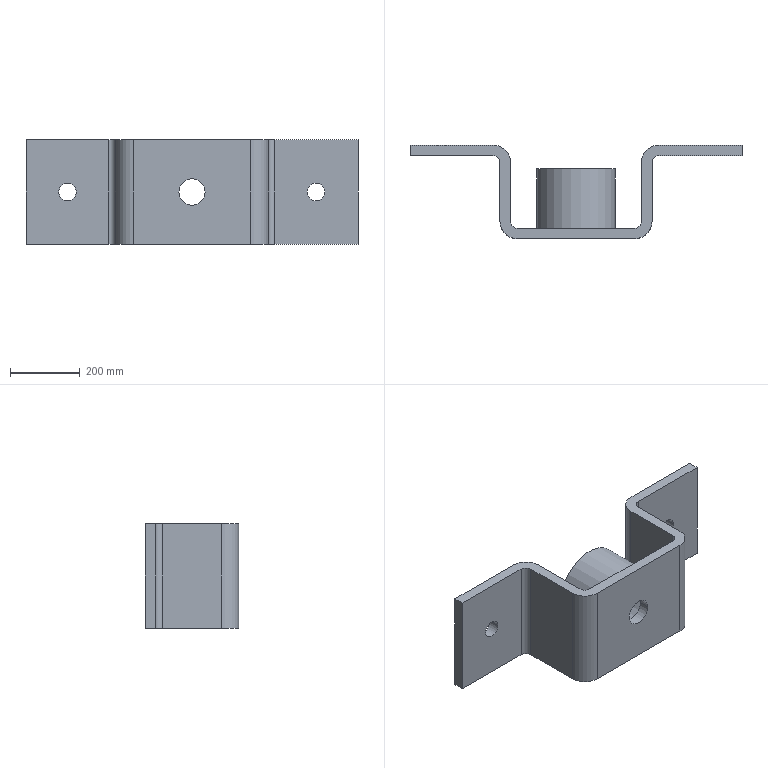Part | SolidWorks | features Fillet 3, ICE 3, Extrusion 1 | 1 solid | 34 faces | box 950 x 268 x 300 mm | volume 14713211 mm3 | cylinder 18 | plane 16 | commonest cylinder face diameters 40 x4 50 x4 100 x4 75 x2 175 x2 225 x2
STEP:
#1=CARTESIAN_POINT('',(330.,208.,150.));
#2=VERTEX_POINT('',#1);
#3=CARTESIAN_POINT('',(380.,208.,150.));
#4=VERTEX_POINT('',#3);
#5=CARTESIAN_POINT('',(355.,208.,150.));
#6=DIRECTION('',(0.,-1.,0.));
#7=DIRECTION('',(0.,0.,1.));
#8=AXIS2_PLACEMENT_3D('',#5,#6,#7);
#9=CIRCLE('',#8,25.);
#10=EDGE_CURVE('',#2,#4,#9,.T.);
#11=ORIENTED_EDGE('',*,*,#10,.T.);
#12=CARTESIAN_POINT('',(380.,238.,150.));
#13=VERTEX_POINT('',#12);
#14=CARTESIAN_POINT('',(380.,-30.001,150.));
#15=DIRECTION('',(0.,1.,0.));
#16=VECTOR('',#15,1000.);
#17=LINE('',#14,#16);
#18=EDGE_CURVE('',#4,#13,#17,.T.);
#19=ORIENTED_EDGE('',*,*,#18,.T.);
#20=CARTESIAN_POINT('',(330.,238.,150.));
#21=VERTEX_POINT('',#20);
#22=CARTESIAN_POINT('',(355.,238.,150.));
#23=DIRECTION('',(0.,1.,0.));
#24=DIRECTION('',(-1.,0.,0.));
#25=AXIS2_PLACEMENT_3D('',#22,#23,#24);
#26=CIRCLE('',#25,25.);
#27=EDGE_CURVE('',#13,#21,#26,.T.);
#28=ORIENTED_EDGE('',*,*,#27,.T.);
#29=CARTESIAN_POINT('',(330.,-30.001,150.));
#30=DIRECTION('',(0.,1.,0.));
#31=VECTOR('',#30,1000.);
#32=LINE('',#29,#31);
#33=EDGE_CURVE('',#2,#21,#32,.T.);
#34=ORIENTED_EDGE('',*,*,#33,.F.);
#35=EDGE_LOOP('',(#11,#19,#28,#34));
#36=FACE_OUTER_BOUND('',#35,.T.);
#37=CARTESIAN_POINT('',(355.,-30.001,150.));
#38=DIRECTION('',(0.,1.,0.));
#39=DIRECTION('',(-1.,0.,0.));
#40=AXIS2_PLACEMENT_3D('',#37,#38,#39);
#41=CYLINDRICAL_SURFACE('',#40,25.);
#42=ADVANCED_FACE('',(#36),#41,.F.);
#43=CARTESIAN_POINT('',(-381.25,208.,150.));
#44=VERTEX_POINT('',#43);
#45=CARTESIAN_POINT('',(-331.25,208.,150.));
#46=VERTEX_POINT('',#45);
#47=CARTESIAN_POINT('',(-356.25,208.,150.));
#48=DIRECTION('',(0.,-1.,0.));
#49=DIRECTION('',(0.,0.,1.));
#50=AXIS2_PLACEMENT_3D('',#47,#48,#49);
#51=CIRCLE('',#50,25.);
#52=EDGE_CURVE('',#44,#46,#51,.T.);
#53=ORIENTED_EDGE('',*,*,#52,.T.);
#54=CARTESIAN_POINT('',(-331.25,238.,150.));
#55=VERTEX_POINT('',#54);
#56=CARTESIAN_POINT('',(-331.25,-30.001,150.));
#57=DIRECTION('',(0.,1.,0.));
#58=VECTOR('',#57,1000.);
#59=LINE('',#56,#58);
#60=EDGE_CURVE('',#46,#55,#59,.T.);
#61=ORIENTED_EDGE('',*,*,#60,.T.);
#62=CARTESIAN_POINT('',(-381.25,238.,150.));
#63=VERTEX_POINT('',#62);
#64=CARTESIAN_POINT('',(-356.25,238.,150.));
#65=DIRECTION('',(0.,1.,0.));
#66=DIRECTION('',(-1.,0.,0.));
#67=AXIS2_PLACEMENT_3D('',#64,#65,#66);
#68=CIRCLE('',#67,25.);
#69=EDGE_CURVE('',#55,#63,#68,.T.);
#70=ORIENTED_EDGE('',*,*,#69,.T.);
#71=CARTESIAN_POINT('',(-381.25,-30.001,150.));
#72=DIRECTION('',(0.,1.,0.));
#73=VECTOR('',#72,1000.);
#74=LINE('',#71,#73);
#75=EDGE_CURVE('',#44,#63,#74,.T.);
#76=ORIENTED_EDGE('',*,*,#75,.F.);
#77=EDGE_LOOP('',(#53,#61,#70,#76));
#78=FACE_OUTER_BOUND('',#77,.T.);
#79=CARTESIAN_POINT('',(-356.25,-30.001,150.));
#80=DIRECTION('',(0.,1.,0.));
#81=DIRECTION('',(-1.,0.,0.));
#82=AXIS2_PLACEMENT_3D('',#79,#80,#81);
#83=CYLINDRICAL_SURFACE('',#82,25.);
#84=ADVANCED_FACE('',(#78),#83,.F.);
#85=CARTESIAN_POINT('',(-37.5,-30.,150.));
#86=VERTEX_POINT('',#85);
#87=CARTESIAN_POINT('',(37.5,-30.,150.));
#88=VERTEX_POINT('',#87);
#89=CARTESIAN_POINT('',(0.,-30.,150.));
#90=DIRECTION('',(0.,-1.,0.));
#91=DIRECTION('',(-1.,0.,0.));
#92=AXIS2_PLACEMENT_3D('',#89,#90,#91);
#93=CIRCLE('',#92,37.5);
#94=EDGE_CURVE('',#86,#88,#93,.T.);
#95=ORIENTED_EDGE('',*,*,#94,.T.);
#96=CARTESIAN_POINT('',(37.5,0.,150.));
#97=VERTEX_POINT('',#96);
#98=CARTESIAN_POINT('',(37.5,-30.001,150.));
#99=DIRECTION('',(0.,1.,0.));
#100=VECTOR('',#99,1000.);
#101=LINE('',#98,#100);
#102=EDGE_CURVE('',#88,#97,#101,.T.);
#103=ORIENTED_EDGE('',*,*,#102,.T.);
#104=CARTESIAN_POINT('',(-37.5,0.,150.));
#105=VERTEX_POINT('',#104);
#106=CARTESIAN_POINT('',(0.,0.,150.));
#107=DIRECTION('',(0.,1.,0.));
#108=DIRECTION('',(-1.,0.,0.));
#109=AXIS2_PLACEMENT_3D('',#106,#107,#108);
#110=CIRCLE('',#109,37.5);
#111=EDGE_CURVE('',#97,#105,#110,.T.);
#112=ORIENTED_EDGE('',*,*,#111,.T.);
#113=CARTESIAN_POINT('',(-37.5,-30.001,150.));
#114=DIRECTION('',(0.,1.,0.));
#115=VECTOR('',#114,1000.);
#116=LINE('',#113,#115);
#117=EDGE_CURVE('',#86,#105,#116,.T.);
#118=ORIENTED_EDGE('',*,*,#117,.F.);
#119=EDGE_LOOP('',(#95,#103,#112,#118));
#120=FACE_OUTER_BOUND('',#119,.T.);
#121=CARTESIAN_POINT('',(0.,-30.001,150.));
#122=DIRECTION('',(0.,1.,0.));
#123=DIRECTION('',(-1.,0.,0.));
#124=AXIS2_PLACEMENT_3D('',#121,#122,#123);
#125=CYLINDRICAL_SURFACE('',#124,37.5);
#126=ADVANCED_FACE('',(#120),#125,.F.);
#127=CARTESIAN_POINT('',(87.5,170.,150.));
#128=VERTEX_POINT('',#127);
#129=CARTESIAN_POINT('',(-87.5,170.,150.));
#130=VERTEX_POINT('',#129);
#131=CARTESIAN_POINT('',(0.,170.,150.));
#132=DIRECTION('',(0.,1.,0.));
#133=DIRECTION('',(-1.,0.,0.));
#134=AXIS2_PLACEMENT_3D('',#131,#132,#133);
#135=CIRCLE('',#134,87.5);
#136=EDGE_CURVE('',#128,#130,#135,.T.);
#137=ORIENTED_EDGE('',*,*,#136,.T.);
#138=CARTESIAN_POINT('',(-87.5,0.,150.));
#139=VERTEX_POINT('',#138);
#140=CARTESIAN_POINT('',(-87.5,170.,150.));
#141=DIRECTION('',(0.,-1.,0.));
#142=VECTOR('',#141,1000.);
#143=LINE('',#140,#142);
#144=EDGE_CURVE('',#130,#139,#143,.T.);
#145=ORIENTED_EDGE('',*,*,#144,.T.);
#146=CARTESIAN_POINT('',(87.5,0.,150.));
#147=VERTEX_POINT('',#146);
#148=CARTESIAN_POINT('',(0.,0.,150.));
#149=DIRECTION('',(0.,1.,0.));
#150=DIRECTION('',(-1.,0.,0.));
#151=AXIS2_PLACEMENT_3D('',#148,#149,#150);
#152=CIRCLE('',#151,87.5);
#153=EDGE_CURVE('',#147,#139,#152,.T.);
#154=ORIENTED_EDGE('',*,*,#153,.F.);
#155=CARTESIAN_POINT('',(87.5,170.,150.));
#156=DIRECTION('',(0.,-1.,0.));
#157=VECTOR('',#156,1000.);
#158=LINE('',#155,#157);
#159=EDGE_CURVE('',#128,#147,#158,.T.);
#160=ORIENTED_EDGE('',*,*,#159,.F.);
#161=EDGE_LOOP('',(#137,#145,#154,#160));
#162=FACE_OUTER_BOUND('',#161,.T.);
#163=CARTESIAN_POINT('',(0.,170.,150.));
#164=DIRECTION('',(0.,-1.,0.));
#165=DIRECTION('',(1.,0.,0.));
#166=AXIS2_PLACEMENT_3D('',#163,#164,#165);
#167=CYLINDRICAL_SURFACE('',#166,87.5);
#168=ADVANCED_FACE('',(#162),#167,.F.);
#169=CARTESIAN_POINT('',(-112.5,170.,150.));
#170=VERTEX_POINT('',#169);
#171=CARTESIAN_POINT('',(112.5,170.,150.));
#172=VERTEX_POINT('',#171);
#173=CARTESIAN_POINT('',(0.,170.,150.));
#174=DIRECTION('',(0.,1.,0.));
#175=DIRECTION('',(-1.,0.,0.));
#176=AXIS2_PLACEMENT_3D('',#173,#174,#175);
#177=CIRCLE('',#176,112.5);
#178=EDGE_CURVE('',#170,#172,#177,.T.);
#179=ORIENTED_EDGE('',*,*,#178,.F.);
#180=CARTESIAN_POINT('',(-112.5,0.,150.));
#181=VERTEX_POINT('',#180);
#182=CARTESIAN_POINT('',(-112.5,170.,150.));
#183=DIRECTION('',(0.,-1.,0.));
#184=VECTOR('',#183,1000.);
#185=LINE('',#182,#184);
#186=EDGE_CURVE('',#170,#181,#185,.T.);
#187=ORIENTED_EDGE('',*,*,#186,.T.);
#188=CARTESIAN_POINT('',(112.5,0.,150.));
#189=VERTEX_POINT('',#188);
#190=CARTESIAN_POINT('',(0.,0.,150.));
#191=DIRECTION('',(0.,1.,0.));
#192=DIRECTION('',(1.,0.,0.));
#193=AXIS2_PLACEMENT_3D('',#190,#191,#192);
#194=CIRCLE('',#193,112.5);
#195=EDGE_CURVE('',#181,#189,#194,.T.);
#196=ORIENTED_EDGE('',*,*,#195,.T.);
#197=CARTESIAN_POINT('',(112.5,170.,150.));
#198=DIRECTION('',(0.,-1.,0.));
#199=VECTOR('',#198,1000.);
#200=LINE('',#197,#199);
#201=EDGE_CURVE('',#172,#189,#200,.T.);
#202=ORIENTED_EDGE('',*,*,#201,.F.);
#203=EDGE_LOOP('',(#179,#187,#196,#202));
#204=FACE_OUTER_BOUND('',#203,.T.);
#205=CARTESIAN_POINT('',(0.,170.,150.));
#206=DIRECTION('',(0.,-1.,0.));
#207=DIRECTION('',(1.,0.,0.));
#208=AXIS2_PLACEMENT_3D('',#205,#206,#207);
#209=CYLINDRICAL_SURFACE('',#208,112.5);
#210=ADVANCED_FACE('',(#204),#209,.T.);
#211=CARTESIAN_POINT('',(167.5,0.,300.));
#212=VERTEX_POINT('',#211);
#213=CARTESIAN_POINT('',(-167.5,0.,300.));
#214=VERTEX_POINT('',#213);
#215=CARTESIAN_POINT('',(187.5,0.,300.));
#216=DIRECTION('',(-1.,0.,0.));
#217=VECTOR('',#216,1000.);
#218=LINE('',#215,#217);
#219=EDGE_CURVE('',#212,#214,#218,.T.);
#220=ORIENTED_EDGE('',*,*,#219,.F.);
#221=CARTESIAN_POINT('',(167.5,0.,0.));
#222=VERTEX_POINT('',#221);
#223=CARTESIAN_POINT('',(167.5,0.,0.));
#224=DIRECTION('',(0.,0.,-1.));
#225=VECTOR('',#224,1000.);
#226=LINE('',#223,#225);
#227=EDGE_CURVE('',#212,#222,#226,.T.);
#228=ORIENTED_EDGE('',*,*,#227,.T.);
#229=CARTESIAN_POINT('',(-167.5,0.,0.));
#230=VERTEX_POINT('',#229);
#231=CARTESIAN_POINT('',(187.5,0.,0.));
#232=DIRECTION('',(-1.,0.,0.));
#233=VECTOR('',#232,1000.);
#234=LINE('',#231,#233);
#235=EDGE_CURVE('',#222,#230,#234,.T.);
#236=ORIENTED_EDGE('',*,*,#235,.T.);
#237=CARTESIAN_POINT('',(-167.5,0.,300.));
#238=DIRECTION('',(0.,0.,1.));
#239=VECTOR('',#238,1000.);
#240=LINE('',#237,#239);
#241=EDGE_CURVE('',#230,#214,#240,.T.);
#242=ORIENTED_EDGE('',*,*,#241,.T.);
#243=EDGE_LOOP('',(#220,#228,#236,#242));
#244=FACE_OUTER_BOUND('',#243,.T.);
#245=CARTESIAN_POINT('',(0.,0.,150.));
#246=DIRECTION('',(0.,1.,0.));
#247=DIRECTION('',(1.,0.,0.));
#248=AXIS2_PLACEMENT_3D('',#245,#246,#247);
#249=CIRCLE('',#248,112.5);
#250=EDGE_CURVE('',#189,#181,#249,.T.);
#251=ORIENTED_EDGE('',*,*,#250,.F.);
#252=ORIENTED_EDGE('',*,*,#195,.F.);
#253=EDGE_LOOP('',(#251,#252));
#254=FACE_BOUND('',#253,.T.);
#255=CARTESIAN_POINT('',(187.5,0.,300.));
#256=DIRECTION('',(0.,-1.,0.));
#257=DIRECTION('',(1.,0.,0.));
#258=AXIS2_PLACEMENT_3D('',#255,#256,#257);
#259=PLANE('',#258);
#260=ADVANCED_FACE('',(#244,#254),#259,.F.);
#261=CARTESIAN_POINT('',(-187.5,20.,0.));
#262=VERTEX_POINT('',#261);
#263=CARTESIAN_POINT('',(-187.5,188.,0.));
#264=VERTEX_POINT('',#263);
#265=CARTESIAN_POINT('',(-187.5,0.,0.));
#266=DIRECTION('',(0.,1.,0.));
#267=VECTOR('',#266,1000.);
#268=LINE('',#265,#267);
#269=EDGE_CURVE('',#262,#264,#268,.T.);
#270=ORIENTED_EDGE('',*,*,#269,.T.);
#271=CARTESIAN_POINT('',(-187.5,188.,300.));
#272=VERTEX_POINT('',#271);
#273=CARTESIAN_POINT('',(-187.5,188.,300.));
#274=DIRECTION('',(0.,0.,1.));
#275=VECTOR('',#274,1000.);
#276=LINE('',#273,#275);
#277=EDGE_CURVE('',#264,#272,#276,.T.);
#278=ORIENTED_EDGE('',*,*,#277,.T.);
#279=CARTESIAN_POINT('',(-187.5,20.,300.));
#280=VERTEX_POINT('',#279);
#281=CARTESIAN_POINT('',(-187.5,0.,300.));
#282=DIRECTION('',(0.,1.,0.));
#283=VECTOR('',#282,1000.);
#284=LINE('',#281,#283);
#285=EDGE_CURVE('',#280,#272,#284,.T.);
#286=ORIENTED_EDGE('',*,*,#285,.F.);
#287=CARTESIAN_POINT('',(-187.5,20.,0.));
#288=DIRECTION('',(0.,0.,-1.));
#289=VECTOR('',#288,1000.);
#290=LINE('',#287,#289);
#291=EDGE_CURVE('',#280,#262,#290,.T.);
#292=ORIENTED_EDGE('',*,*,#291,.T.);
#293=EDGE_LOOP('',(#270,#278,#286,#292));
#294=FACE_OUTER_BOUND('',#293,.T.);
#295=CARTESIAN_POINT('',(-187.5,0.,300.));
#296=DIRECTION('',(-1.,0.,0.));
#297=DIRECTION('',(0.,0.,1.));
#298=AXIS2_PLACEMENT_3D('',#295,#296,#297);
#299=PLANE('',#298);
#300=ADVANCED_FACE('',(#294),#299,.F.);
#301=CARTESIAN_POINT('',(-356.25,238.,150.));
#302=DIRECTION('',(0.,1.,0.));
#303=DIRECTION('',(-1.,0.,0.));
#304=AXIS2_PLACEMENT_3D('',#301,#302,#303);
#305=CIRCLE('',#304,25.);
#306=EDGE_CURVE('',#63,#55,#305,.T.);
#307=ORIENTED_EDGE('',*,*,#306,.F.);
#308=ORIENTED_EDGE('',*,*,#69,.F.);
#309=EDGE_LOOP('',(#307,#308));
#310=FACE_BOUND('',#309,.T.);
#311=CARTESIAN_POINT('',(-237.5,238.,300.));
#312=VERTEX_POINT('',#311);
#313=CARTESIAN_POINT('',(-475.,238.,300.));
#314=VERTEX_POINT('',#313);
#315=CARTESIAN_POINT('',(-187.5,238.,300.));
#316=DIRECTION('',(-1.,0.,0.));
#317=VECTOR('',#316,1000.);
#318=LINE('',#315,#317);
#319=EDGE_CURVE('',#312,#314,#318,.T.);
#320=ORIENTED_EDGE('',*,*,#319,.F.);
#321=CARTESIAN_POINT('',(-237.5,238.,0.));
#322=VERTEX_POINT('',#321);
#323=CARTESIAN_POINT('',(-237.5,238.,300.));
#324=DIRECTION('',(0.,0.,-1.));
#325=VECTOR('',#324,1000.);
#326=LINE('',#323,#325);
#327=EDGE_CURVE('',#312,#322,#326,.T.);
#328=ORIENTED_EDGE('',*,*,#327,.T.);
#329=CARTESIAN_POINT('',(-475.,238.,0.));
#330=VERTEX_POINT('',#329);
#331=CARTESIAN_POINT('',(-187.5,238.,0.));
#332=DIRECTION('',(-1.,0.,0.));
#333=VECTOR('',#332,1000.);
#334=LINE('',#331,#333);
#335=EDGE_CURVE('',#322,#330,#334,.T.);
#336=ORIENTED_EDGE('',*,*,#335,.T.);
#337=CARTESIAN_POINT('',(-475.,238.,300.));
#338=DIRECTION('',(0.,0.,-1.));
#339=VECTOR('',#338,1000.);
#340=LINE('',#337,#339);
#341=EDGE_CURVE('',#314,#330,#340,.T.);
#342=ORIENTED_EDGE('',*,*,#341,.F.);
#343=EDGE_LOOP('',(#320,#328,#336,#342));
#344=FACE_OUTER_BOUND('',#343,.T.);
#345=CARTESIAN_POINT('',(-187.5,238.,300.));
#346=DIRECTION('',(0.,-1.,0.));
#347=DIRECTION('',(1.,0.,0.));
#348=AXIS2_PLACEMENT_3D('',#345,#346,#347);
#349=PLANE('',#348);
#350=ADVANCED_FACE('',(#310,#344),#349,.F.);
#351=CARTESIAN_POINT('',(-475.,208.,0.));
#352=VERTEX_POINT('',#351);
#353=CARTESIAN_POINT('',(-475.,238.,0.));
#354=DIRECTION('',(0.,-1.,0.));
#355=VECTOR('',#354,1000.);
#356=LINE('',#353,#355);
#357=EDGE_CURVE('',#330,#352,#356,.T.);
#358=ORIENTED_EDGE('',*,*,#357,.T.);
#359=CARTESIAN_POINT('',(-475.,208.,300.));
#360=VERTEX_POINT('',#359);
#361=CARTESIAN_POINT('',(-475.,208.,300.));
#362=DIRECTION('',(0.,0.,-1.));
#363=VECTOR('',#362,1000.);
#364=LINE('',#361,#363);
#365=EDGE_CURVE('',#360,#352,#364,.T.);
#366=ORIENTED_EDGE('',*,*,#365,.F.);
#367=CARTESIAN_POINT('',(-475.,238.,300.));
#368=DIRECTION('',(0.,-1.,0.));
#369=VECTOR('',#368,1000.);
#370=LINE('',#367,#369);
#371=EDGE_CURVE('',#314,#360,#370,.T.);
#372=ORIENTED_EDGE('',*,*,#371,.F.);
#373=ORIENTED_EDGE('',*,*,#341,.T.);
#374=EDGE_LOOP('',(#358,#366,#372,#373));
#375=FACE_OUTER_BOUND('',#374,.T.);
#376=CARTESIAN_POINT('',(-475.,238.,300.));
#377=DIRECTION('',(1.,0.,0.));
#378=DIRECTION('',(0.,0.,-1.));
#379=AXIS2_PLACEMENT_3D('',#376,#377,#378);
#380=PLANE('',#379);
#381=ADVANCED_FACE('',(#375),#380,.F.);
#382=ORIENTED_EDGE('',*,*,#52,.F.);
#383=CARTESIAN_POINT('',(-356.25,208.,150.));
#384=DIRECTION('',(0.,-1.,0.));
#385=DIRECTION('',(0.,0.,1.));
#386=AXIS2_PLACEMENT_3D('',#383,#384,#385);
#387=CIRCLE('',#386,25.);
#388=EDGE_CURVE('',#46,#44,#387,.T.);
#389=ORIENTED_EDGE('',*,*,#388,.F.);
#390=EDGE_LOOP('',(#382,#389));
#391=FACE_BOUND('',#390,.T.);
#392=CARTESIAN_POINT('',(-237.5,208.,0.));
#393=VERTEX_POINT('',#392);
#394=CARTESIAN_POINT('',(-475.,208.,0.));
#395=DIRECTION('',(1.,0.,0.));
#396=VECTOR('',#395,1000.);
#397=LINE('',#394,#396);
#398=EDGE_CURVE('',#352,#393,#397,.T.);
#399=ORIENTED_EDGE('',*,*,#398,.T.);
#400=CARTESIAN_POINT('',(-237.5,208.,300.));
#401=VERTEX_POINT('',#400);
#402=CARTESIAN_POINT('',(-237.5,208.,300.));
#403=DIRECTION('',(0.,0.,1.));
#404=VECTOR('',#403,1000.);
#405=LINE('',#402,#404);
#406=EDGE_CURVE('',#393,#401,#405,.T.);
#407=ORIENTED_EDGE('',*,*,#406,.T.);
#408=CARTESIAN_POINT('',(-475.,208.,300.));
#409=DIRECTION('',(1.,0.,0.));
#410=VECTOR('',#409,1000.);
#411=LINE('',#408,#410);
#412=EDGE_CURVE('',#360,#401,#411,.T.);
#413=ORIENTED_EDGE('',*,*,#412,.F.);
#414=ORIENTED_EDGE('',*,*,#365,.T.);
#415=EDGE_LOOP('',(#399,#407,#413,#414));
#416=FACE_OUTER_BOUND('',#415,.T.);
#417=CARTESIAN_POINT('',(-475.,208.,300.));
#418=DIRECTION('',(0.,1.,0.));
#419=DIRECTION('',(0.,0.,1.));
#420=AXIS2_PLACEMENT_3D('',#417,#418,#419);
#421=PLANE('',#420);
#422=ADVANCED_FACE('',(#391,#416),#421,.F.);
#423=CARTESIAN_POINT('',(-217.5,188.,300.));
#424=VERTEX_POINT('',#423);
#425=CARTESIAN_POINT('',(-217.5,20.,300.));
#426=VERTEX_POINT('',#425);
#427=CARTESIAN_POINT('',(-217.5,208.,300.));
#428=DIRECTION('',(0.,-1.,0.));
#429=VECTOR('',#428,1000.);
#430=LINE('',#427,#429);
#431=EDGE_CURVE('',#424,#426,#430,.T.);
#432=ORIENTED_EDGE('',*,*,#431,.F.);
#433=CARTESIAN_POINT('',(-217.5,188.,0.));
#434=VERTEX_POINT('',#433);
#435=CARTESIAN_POINT('',(-217.5,188.,0.));
#436=DIRECTION('',(0.,0.,-1.));
#437=VECTOR('',#436,1000.);
#438=LINE('',#435,#437);
#439=EDGE_CURVE('',#424,#434,#438,.T.);
#440=ORIENTED_EDGE('',*,*,#439,.T.);
#441=CARTESIAN_POINT('',(-217.5,20.,0.));
#442=VERTEX_POINT('',#441);
#443=CARTESIAN_POINT('',(-217.5,208.,0.));
#444=DIRECTION('',(0.,-1.,0.));
#445=VECTOR('',#444,1000.);
#446=LINE('',#443,#445);
#447=EDGE_CURVE('',#434,#442,#446,.T.);
#448=ORIENTED_EDGE('',*,*,#447,.T.);
#449=CARTESIAN_POINT('',(-217.5,20.,300.));
#450=DIRECTION('',(0.,0.,1.));
#451=VECTOR('',#450,1000.);
#452=LINE('',#449,#451);
#453=EDGE_CURVE('',#442,#426,#452,.T.);
#454=ORIENTED_EDGE('',*,*,#453,.T.);
#455=EDGE_LOOP('',(#432,#440,#448,#454));
#456=FACE_OUTER_BOUND('',#455,.T.);
#457=CARTESIAN_POINT('',(-217.5,208.,300.));
#458=DIRECTION('',(1.,0.,0.));
#459=DIRECTION('',(0.,1.,0.));
#460=AXIS2_PLACEMENT_3D('',#457,#458,#459);
#461=PLANE('',#460);
#462=ADVANCED_FACE('',(#456),#461,.F.);
#463=ORIENTED_EDGE('',*,*,#94,.F.);
#464=CARTESIAN_POINT('',(0.,-30.,150.));
#465=DIRECTION('',(0.,-1.,0.));
#466=DIRECTION('',(-1.,0.,0.));
#467=AXIS2_PLACEMENT_3D('',#464,#465,#466);
#468=CIRCLE('',#467,37.5);
#469=EDGE_CURVE('',#88,#86,#468,.T.);
#470=ORIENTED_EDGE('',*,*,#469,.F.);
#471=EDGE_LOOP('',(#463,#470));
#472=FACE_BOUND('',#471,.T.);
#473=CARTESIAN_POINT('',(-167.5,-30.,0.));
#474=VERTEX_POINT('',#473);
#475=CARTESIAN_POINT('',(167.5,-30.,0.));
#476=VERTEX_POINT('',#475);
#477=CARTESIAN_POINT('',(-217.5,-30.,0.));
#478=DIRECTION('',(1.,0.,0.));
#479=VECTOR('',#478,1000.);
#480=LINE('',#477,#479);
#481=EDGE_CURVE('',#474,#476,#480,.T.);
#482=ORIENTED_EDGE('',*,*,#481,.T.);
#483=CARTESIAN_POINT('',(167.5,-30.,300.));
#484=VERTEX_POINT('',#483);
#485=CARTESIAN_POINT('',(167.5,-30.,300.));
#486=DIRECTION('',(0.,0.,1.));
#487=VECTOR('',#486,1000.);
#488=LINE('',#485,#487);
#489=EDGE_CURVE('',#476,#484,#488,.T.);
#490=ORIENTED_EDGE('',*,*,#489,.T.);
#491=CARTESIAN_POINT('',(-167.5,-30.,300.));
#492=VERTEX_POINT('',#491);
#493=CARTESIAN_POINT('',(-217.5,-30.,300.));
#494=DIRECTION('',(1.,0.,0.));
#495=VECTOR('',#494,1000.);
#496=LINE('',#493,#495);
#497=EDGE_CURVE('',#492,#484,#496,.T.);
#498=ORIENTED_EDGE('',*,*,#497,.F.);
#499=CARTESIAN_POINT('',(-167.5,-30.,300.));
#500=DIRECTION('',(0.,0.,-1.));
#501=VECTOR('',#500,1000.);
#502=LINE('',#499,#501);
#503=EDGE_CURVE('',#492,#474,#502,.T.);
#504=ORIENTED_EDGE('',*,*,#503,.T.);
#505=EDGE_LOOP('',(#482,#490,#498,#504));
#506=FACE_OUTER_BOUND('',#505,.T.);
#507=CARTESIAN_POINT('',(-217.5,-30.,300.));
#508=DIRECTION('',(0.,1.,0.));
#509=DIRECTION('',(-1.,0.,0.));
#510=AXIS2_PLACEMENT_3D('',#507,#508,#509);
#511=PLANE('',#510);
#512=ADVANCED_FACE('',(#472,#506),#511,.F.);
#513=CARTESIAN_POINT('',(217.5,20.,0.));
#514=VERTEX_POINT('',#513);
#515=CARTESIAN_POINT('',(217.5,188.,0.));
#516=VERTEX_POINT('',#515);
#517=CARTESIAN_POINT('',(217.5,208.,0.));
#518=DIRECTION('',(0.,1.,0.));
#519=VECTOR('',#518,1000.);
#520=LINE('',#517,#519);
#521=EDGE_CURVE('',#514,#516,#520,.T.);
#522=ORIENTED_EDGE('',*,*,#521,.T.);
#523=CARTESIAN_POINT('',(217.5,188.,300.));
#524=VERTEX_POINT('',#523);
#525=CARTESIAN_POINT('',(217.5,188.,300.));
#526=DIRECTION('',(0.,0.,1.));
#527=VECTOR('',#526,1000.);
#528=LINE('',#525,#527);
#529=EDGE_CURVE('',#516,#524,#528,.T.);
#530=ORIENTED_EDGE('',*,*,#529,.T.);
#531=CARTESIAN_POINT('',(217.5,20.,300.));
#532=VERTEX_POINT('',#531);
#533=CARTESIAN_POINT('',(217.5,208.,300.));
#534=DIRECTION('',(0.,1.,0.));
#535=VECTOR('',#534,1000.);
#536=LINE('',#533,#535);
#537=EDGE_CURVE('',#532,#524,#536,.T.);
#538=ORIENTED_EDGE('',*,*,#537,.F.);
#539=CARTESIAN_POINT('',(217.5,20.,300.));
#540=DIRECTION('',(0.,0.,-1.));
#541=VECTOR('',#540,1000.);
#542=LINE('',#539,#541);
#543=EDGE_CURVE('',#532,#514,#542,.T.);
#544=ORIENTED_EDGE('',*,*,#543,.T.);
#545=EDGE_LOOP('',(#522,#530,#538,#544));
#546=FACE_OUTER_BOUND('',#545,.T.);
#547=CARTESIAN_POINT('',(217.5,208.,300.));
#548=DIRECTION('',(-1.,0.,0.));
#549=DIRECTION('',(0.,-1.,0.));
#550=AXIS2_PLACEMENT_3D('',#547,#548,#549);
#551=PLANE('',#550);
#552=ADVANCED_FACE('',(#546),#551,.F.);
#553=ORIENTED_EDGE('',*,*,#10,.F.);
#554=CARTESIAN_POINT('',(355.,208.,150.));
#555=DIRECTION('',(0.,-1.,0.));
#556=DIRECTION('',(0.,0.,1.));
#557=AXIS2_PLACEMENT_3D('',#554,#555,#556);
#558=CIRCLE('',#557,25.);
#559=EDGE_CURVE('',#4,#2,#558,.T.);
#560=ORIENTED_EDGE('',*,*,#559,.F.);
#561=EDGE_LOOP('',(#553,#560));
#562=FACE_BOUND('',#561,.T.);
#563=CARTESIAN_POINT('',(237.5,208.,300.));
#564=VERTEX_POINT('',#563);
#565=CARTESIAN_POINT('',(475.,208.,300.));
#566=VERTEX_POINT('',#565);
#567=CARTESIAN_POINT('',(475.,208.,300.));
#568=DIRECTION('',(1.,0.,0.));
#569=VECTOR('',#568,1000.);
#570=LINE('',#567,#569);
#571=EDGE_CURVE('',#564,#566,#570,.T.);
#572=ORIENTED_EDGE('',*,*,#571,.F.);
#573=CARTESIAN_POINT('',(237.5,208.,0.));
#574=VERTEX_POINT('',#573);
#575=CARTESIAN_POINT('',(237.5,208.,0.));
#576=DIRECTION('',(0.,0.,-1.));
#577=VECTOR('',#576,1000.);
#578=LINE('',#575,#577);
#579=EDGE_CURVE('',#564,#574,#578,.T.);
#580=ORIENTED_EDGE('',*,*,#579,.T.);
#581=CARTESIAN_POINT('',(475.,208.,0.));
#582=VERTEX_POINT('',#581);
#583=CARTESIAN_POINT('',(475.,208.,0.));
#584=DIRECTION('',(1.,0.,0.));
#585=VECTOR('',#584,1000.);
#586=LINE('',#583,#585);
#587=EDGE_CURVE('',#574,#582,#586,.T.);
#588=ORIENTED_EDGE('',*,*,#587,.T.);
#589=CARTESIAN_POINT('',(475.,208.,300.));
#590=DIRECTION('',(0.,0.,-1.));
#591=VECTOR('',#590,1000.);
#592=LINE('',#589,#591);
#593=EDGE_CURVE('',#566,#582,#592,.T.);
#594=ORIENTED_EDGE('',*,*,#593,.F.);
#595=EDGE_LOOP('',(#572,#580,#588,#594));
#596=FACE_OUTER_BOUND('',#595,.T.);
#597=CARTESIAN_POINT('',(475.,208.,300.));
#598=DIRECTION('',(0.,1.,0.));
#599=DIRECTION('',(0.,0.,1.));
#600=AXIS2_PLACEMENT_3D('',#597,#598,#599);
#601=PLANE('',#600);
#602=ADVANCED_FACE('',(#562,#596),#601,.F.);
#603=CARTESIAN_POINT('',(475.,238.,0.));
#604=VERTEX_POINT('',#603);
#605=CARTESIAN_POINT('',(475.,238.,0.));
#606=DIRECTION('',(0.,1.,0.));
#607=VECTOR('',#606,1000.);
#608=LINE('',#605,#607);
#609=EDGE_CURVE('',#582,#604,#608,.T.);
#610=ORIENTED_EDGE('',*,*,#609,.T.);
#611=CARTESIAN_POINT('',(475.,238.,300.));
#612=VERTEX_POINT('',#611);
#613=CARTESIAN_POINT('',(475.,238.,300.));
#614=DIRECTION('',(0.,0.,-1.));
#615=VECTOR('',#614,1000.);
#616=LINE('',#613,#615);
#617=EDGE_CURVE('',#612,#604,#616,.T.);
#618=ORIENTED_EDGE('',*,*,#617,.F.);
#619=CARTESIAN_POINT('',(475.,238.,300.));
#620=DIRECTION('',(0.,1.,0.));
#621=VECTOR('',#620,1000.);
#622=LINE('',#619,#621);
#623=EDGE_CURVE('',#566,#612,#622,.T.);
#624=ORIENTED_EDGE('',*,*,#623,.F.);
#625=ORIENTED_EDGE('',*,*,#593,.T.);
#626=EDGE_LOOP('',(#610,#618,#624,#625));
#627=FACE_OUTER_BOUND('',#626,.T.);
#628=CARTESIAN_POINT('',(475.,238.,300.));
#629=DIRECTION('',(-1.,0.,0.));
#630=DIRECTION('',(0.,0.,1.));
#631=AXIS2_PLACEMENT_3D('',#628,#629,#630);
#632=PLANE('',#631);
#633=ADVANCED_FACE('',(#627),#632,.F.);
#634=CARTESIAN_POINT('',(355.,238.,150.));
#635=DIRECTION('',(0.,1.,0.));
#636=DIRECTION('',(-1.,0.,0.));
#637=AXIS2_PLACEMENT_3D('',#634,#635,#636);
#638=CIRCLE('',#637,25.);
#639=EDGE_CURVE('',#21,#13,#638,.T.);
#640=ORIENTED_EDGE('',*,*,#639,.F.);
#641=ORIENTED_EDGE('',*,*,#27,.F.);
#642=EDGE_LOOP('',(#640,#641));
#643=FACE_BOUND('',#642,.T.);
#644=CARTESIAN_POINT('',(237.5,238.,0.));
#645=VERTEX_POINT('',#644);
#646=CARTESIAN_POINT('',(187.5,238.,0.));
#647=DIRECTION('',(-1.,0.,0.));
#648=VECTOR('',#647,1000.);
#649=LINE('',#646,#648);
#650=EDGE_CURVE('',#604,#645,#649,.T.);
#651=ORIENTED_EDGE('',*,*,#650,.T.);
#652=CARTESIAN_POINT('',(237.5,238.,300.));
#653=VERTEX_POINT('',#652);
#654=CARTESIAN_POINT('',(237.5,238.,300.));
#655=DIRECTION('',(0.,0.,1.));
#656=VECTOR('',#655,1000.);
#657=LINE('',#654,#656);
#658=EDGE_CURVE('',#645,#653,#657,.T.);
#659=ORIENTED_EDGE('',*,*,#658,.T.);
#660=CARTESIAN_POINT('',(187.5,238.,300.));
#661=DIRECTION('',(-1.,0.,0.));
#662=VECTOR('',#661,1000.);
#663=LINE('',#660,#662);
#664=EDGE_CURVE('',#612,#653,#663,.T.);
#665=ORIENTED_EDGE('',*,*,#664,.F.);
#666=ORIENTED_EDGE('',*,*,#617,.T.);
#667=EDGE_LOOP('',(#651,#659,#665,#666));
#668=FACE_OUTER_BOUND('',#667,.T.);
#669=CARTESIAN_POINT('',(187.5,238.,300.));
#670=DIRECTION('',(0.,-1.,0.));
#671=DIRECTION('',(1.,0.,0.));
#672=AXIS2_PLACEMENT_3D('',#669,#670,#671);
#673=PLANE('',#672);
#674=ADVANCED_FACE('',(#643,#668),#673,.F.);
#675=CARTESIAN_POINT('',(187.5,188.,300.));
#676=VERTEX_POINT('',#675);
#677=CARTESIAN_POINT('',(187.5,20.,300.));
#678=VERTEX_POINT('',#677);
#679=CARTESIAN_POINT('',(187.5,0.,300.));
#680=DIRECTION('',(0.,-1.,0.));
#681=VECTOR('',#680,1000.);
#682=LINE('',#679,#681);
#683=EDGE_CURVE('',#676,#678,#682,.T.);
#684=ORIENTED_EDGE('',*,*,#683,.F.);
#685=CARTESIAN_POINT('',(187.5,188.,0.));
#686=VERTEX_POINT('',#685);
#687=CARTESIAN_POINT('',(187.5,188.,300.));
#688=DIRECTION('',(0.,0.,-1.));
#689=VECTOR('',#688,1000.);
#690=LINE('',#687,#689);
#691=EDGE_CURVE('',#676,#686,#690,.T.);
#692=ORIENTED_EDGE('',*,*,#691,.T.);
#693=CARTESIAN_POINT('',(187.5,20.,0.));
#694=VERTEX_POINT('',#693);
#695=CARTESIAN_POINT('',(187.5,0.,0.));
#696=DIRECTION('',(0.,-1.,0.));
#697=VECTOR('',#696,1000.);
#698=LINE('',#695,#697);
#699=EDGE_CURVE('',#686,#694,#698,.T.);
#700=ORIENTED_EDGE('',*,*,#699,.T.);
#701=CARTESIAN_POINT('',(187.5,20.,300.));
#702=DIRECTION('',(0.,0.,1.));
#703=VECTOR('',#702,1000.);
#704=LINE('',#701,#703);
#705=EDGE_CURVE('',#694,#678,#704,.T.);
#706=ORIENTED_EDGE('',*,*,#705,.T.);
#707=EDGE_LOOP('',(#684,#692,#700,#706));
#708=FACE_OUTER_BOUND('',#707,.T.);
#709=CARTESIAN_POINT('',(187.5,0.,300.));
#710=DIRECTION('',(1.,0.,0.));
#711=DIRECTION('',(0.,0.,-1.));
#712=AXIS2_PLACEMENT_3D('',#709,#710,#711);
#713=PLANE('',#712);
#714=ADVANCED_FACE('',(#708),#713,.F.);
#715=ORIENTED_EDGE('',*,*,#497,.T.);
#716=CARTESIAN_POINT('',(167.5,20.,300.));
#717=DIRECTION('',(0.,0.,1.));
#718=DIRECTION('',(1.,0.,0.));
#719=AXIS2_PLACEMENT_3D('',#716,#717,#718);
#720=CIRCLE('',#719,50.);
#721=EDGE_CURVE('',#484,#532,#720,.T.);
#722=ORIENTED_EDGE('',*,*,#721,.T.);
#723=ORIENTED_EDGE('',*,*,#537,.T.);
#724=CARTESIAN_POINT('',(237.5,188.,300.));
#725=DIRECTION('',(0.,0.,-1.));
#726=DIRECTION('',(1.,0.,0.));
#727=AXIS2_PLACEMENT_3D('',#724,#725,#726);
#728=CIRCLE('',#727,20.);
#729=EDGE_CURVE('',#524,#564,#728,.T.);
#730=ORIENTED_EDGE('',*,*,#729,.T.);
#731=ORIENTED_EDGE('',*,*,#571,.T.);
#732=ORIENTED_EDGE('',*,*,#623,.T.);
#733=ORIENTED_EDGE('',*,*,#664,.T.);
#734=CARTESIAN_POINT('',(237.5,188.,300.));
#735=DIRECTION('',(0.,0.,1.));
#736=DIRECTION('',(1.,0.,0.));
#737=AXIS2_PLACEMENT_3D('',#734,#735,#736);
#738=CIRCLE('',#737,50.);
#739=EDGE_CURVE('',#653,#676,#738,.T.);
#740=ORIENTED_EDGE('',*,*,#739,.T.);
#741=ORIENTED_EDGE('',*,*,#683,.T.);
#742=CARTESIAN_POINT('',(167.5,20.,300.));
#743=DIRECTION('',(0.,0.,-1.));
#744=DIRECTION('',(1.,0.,0.));
#745=AXIS2_PLACEMENT_3D('',#742,#743,#744);
#746=CIRCLE('',#745,20.);
#747=EDGE_CURVE('',#678,#212,#746,.T.);
#748=ORIENTED_EDGE('',*,*,#747,.T.);
#749=ORIENTED_EDGE('',*,*,#219,.T.);
#750=CARTESIAN_POINT('',(-167.5,20.,300.));
#751=DIRECTION('',(0.,0.,-1.));
#752=DIRECTION('',(1.,0.,0.));
#753=AXIS2_PLACEMENT_3D('',#750,#751,#752);
#754=CIRCLE('',#753,20.);
#755=EDGE_CURVE('',#214,#280,#754,.T.);
#756=ORIENTED_EDGE('',*,*,#755,.T.);
#757=ORIENTED_EDGE('',*,*,#285,.T.);
#758=CARTESIAN_POINT('',(-237.5,188.,300.));
#759=DIRECTION('',(0.,0.,1.));
#760=DIRECTION('',(1.,0.,0.));
#761=AXIS2_PLACEMENT_3D('',#758,#759,#760);
#762=CIRCLE('',#761,50.);
#763=EDGE_CURVE('',#272,#312,#762,.T.);
#764=ORIENTED_EDGE('',*,*,#763,.T.);
#765=ORIENTED_EDGE('',*,*,#319,.T.);
#766=ORIENTED_EDGE('',*,*,#371,.T.);
#767=ORIENTED_EDGE('',*,*,#412,.T.);
#768=CARTESIAN_POINT('',(-237.5,188.,300.));
#769=DIRECTION('',(0.,0.,-1.));
#770=DIRECTION('',(1.,0.,0.));
#771=AXIS2_PLACEMENT_3D('',#768,#769,#770);
#772=CIRCLE('',#771,20.);
#773=EDGE_CURVE('',#401,#424,#772,.T.);
#774=ORIENTED_EDGE('',*,*,#773,.T.);
#775=ORIENTED_EDGE('',*,*,#431,.T.);
#776=CARTESIAN_POINT('',(-167.5,20.,300.));
#777=DIRECTION('',(0.,0.,1.));
#778=DIRECTION('',(1.,0.,0.));
#779=AXIS2_PLACEMENT_3D('',#776,#777,#778);
#780=CIRCLE('',#779,50.);
#781=EDGE_CURVE('',#426,#492,#780,.T.);
#782=ORIENTED_EDGE('',*,*,#781,.T.);
#783=EDGE_LOOP('',(#715,#722,#723,#730,#731,#732,#733,#740,#741,#748,#749,#756,#757,#764,#765,#766,#767,#774,#775,#782));
#784=FACE_OUTER_BOUND('',#783,.T.);
#785=CARTESIAN_POINT('',(0.,0.,300.));
#786=DIRECTION('',(0.,0.,1.));
#787=DIRECTION('',(1.,0.,0.));
#788=AXIS2_PLACEMENT_3D('',#785,#786,#787);
#789=PLANE('',#788);
#790=ADVANCED_FACE('',(#784),#789,.T.);
#791=ORIENTED_EDGE('',*,*,#521,.F.);
#792=CARTESIAN_POINT('',(167.5,20.,0.));
#793=DIRECTION('',(0.,0.,-1.));
#794=DIRECTION('',(1.,0.,0.));
#795=AXIS2_PLACEMENT_3D('',#792,#793,#794);
#796=CIRCLE('',#795,50.);
#797=EDGE_CURVE('',#514,#476,#796,.T.);
#798=ORIENTED_EDGE('',*,*,#797,.T.);
#799=ORIENTED_EDGE('',*,*,#481,.F.);
#800=CARTESIAN_POINT('',(-167.5,20.,0.));
#801=DIRECTION('',(0.,0.,-1.));
#802=DIRECTION('',(1.,0.,0.));
#803=AXIS2_PLACEMENT_3D('',#800,#801,#802);
#804=CIRCLE('',#803,50.);
#805=EDGE_CURVE('',#474,#442,#804,.T.);
#806=ORIENTED_EDGE('',*,*,#805,.T.);
#807=ORIENTED_EDGE('',*,*,#447,.F.);
#808=CARTESIAN_POINT('',(-237.5,188.,0.));
#809=DIRECTION('',(0.,0.,1.));
#810=DIRECTION('',(1.,0.,0.));
#811=AXIS2_PLACEMENT_3D('',#808,#809,#810);
#812=CIRCLE('',#811,20.);
#813=EDGE_CURVE('',#434,#393,#812,.T.);
#814=ORIENTED_EDGE('',*,*,#813,.T.);
#815=ORIENTED_EDGE('',*,*,#398,.F.);
#816=ORIENTED_EDGE('',*,*,#357,.F.);
#817=ORIENTED_EDGE('',*,*,#335,.F.);
#818=CARTESIAN_POINT('',(-237.5,188.,0.));
#819=DIRECTION('',(0.,0.,-1.));
#820=DIRECTION('',(1.,0.,0.));
#821=AXIS2_PLACEMENT_3D('',#818,#819,#820);
#822=CIRCLE('',#821,50.);
#823=EDGE_CURVE('',#322,#264,#822,.T.);
#824=ORIENTED_EDGE('',*,*,#823,.T.);
#825=ORIENTED_EDGE('',*,*,#269,.F.);
#826=CARTESIAN_POINT('',(-167.5,20.,0.));
#827=DIRECTION('',(0.,0.,1.));
#828=DIRECTION('',(1.,0.,0.));
#829=AXIS2_PLACEMENT_3D('',#826,#827,#828);
#830=CIRCLE('',#829,20.);
#831=EDGE_CURVE('',#262,#230,#830,.T.);
#832=ORIENTED_EDGE('',*,*,#831,.T.);
#833=ORIENTED_EDGE('',*,*,#235,.F.);
#834=CARTESIAN_POINT('',(167.5,20.,0.));
#835=DIRECTION('',(0.,0.,1.));
#836=DIRECTION('',(1.,0.,0.));
#837=AXIS2_PLACEMENT_3D('',#834,#835,#836);
#838=CIRCLE('',#837,20.);
#839=EDGE_CURVE('',#222,#694,#838,.T.);
#840=ORIENTED_EDGE('',*,*,#839,.T.);
#841=ORIENTED_EDGE('',*,*,#699,.F.);
#842=CARTESIAN_POINT('',(237.5,188.,0.));
#843=DIRECTION('',(0.,0.,-1.));
#844=DIRECTION('',(1.,0.,0.));
#845=AXIS2_PLACEMENT_3D('',#842,#843,#844);
#846=CIRCLE('',#845,50.);
#847=EDGE_CURVE('',#686,#645,#846,.T.);
#848=ORIENTED_EDGE('',*,*,#847,.T.);
#849=ORIENTED_EDGE('',*,*,#650,.F.);
#850=ORIENTED_EDGE('',*,*,#609,.F.);
#851=ORIENTED_EDGE('',*,*,#587,.F.);
#852=CARTESIAN_POINT('',(237.5,188.,0.));
#853=DIRECTION('',(0.,0.,1.));
#854=DIRECTION('',(1.,0.,0.));
#855=AXIS2_PLACEMENT_3D('',#852,#853,#854);
#856=CIRCLE('',#855,20.);
#857=EDGE_CURVE('',#574,#516,#856,.T.);
#858=ORIENTED_EDGE('',*,*,#857,.T.);
#859=EDGE_LOOP('',(#791,#798,#799,#806,#807,#814,#815,#816,#817,#824,#825,#832,#833,#840,#841,#848,#849,#850,#851,#858));
#860=FACE_OUTER_BOUND('',#859,.T.);
#861=CARTESIAN_POINT('',(0.,0.,0.));
#862=DIRECTION('',(0.,0.,1.));
#863=DIRECTION('',(1.,0.,0.));
#864=AXIS2_PLACEMENT_3D('',#861,#862,#863);
#865=PLANE('',#864);
#866=ADVANCED_FACE('',(#860),#865,.F.);
#867=ORIENTED_EDGE('',*,*,#747,.F.);
#868=ORIENTED_EDGE('',*,*,#705,.F.);
#869=ORIENTED_EDGE('',*,*,#839,.F.);
#870=ORIENTED_EDGE('',*,*,#227,.F.);
#871=EDGE_LOOP('',(#867,#868,#869,#870));
#872=FACE_OUTER_BOUND('',#871,.T.);
#873=CARTESIAN_POINT('',(167.5,20.,300.));
#874=DIRECTION('',(0.,0.,1.));
#875=DIRECTION('',(1.,0.,0.));
#876=AXIS2_PLACEMENT_3D('',#873,#874,#875);
#877=CYLINDRICAL_SURFACE('',#876,20.);
#878=ADVANCED_FACE('',(#872),#877,.F.);
#879=ORIENTED_EDGE('',*,*,#755,.F.);
#880=ORIENTED_EDGE('',*,*,#241,.F.);
#881=ORIENTED_EDGE('',*,*,#831,.F.);
#882=ORIENTED_EDGE('',*,*,#291,.F.);
#883=EDGE_LOOP('',(#879,#880,#881,#882));
#884=FACE_OUTER_BOUND('',#883,.T.);
#885=CARTESIAN_POINT('',(-167.5,20.,300.));
#886=DIRECTION('',(0.,0.,1.));
#887=DIRECTION('',(1.,0.,0.));
#888=AXIS2_PLACEMENT_3D('',#885,#886,#887);
#889=CYLINDRICAL_SURFACE('',#888,20.);
#890=ADVANCED_FACE('',(#884),#889,.F.);
#891=ORIENTED_EDGE('',*,*,#721,.F.);
#892=ORIENTED_EDGE('',*,*,#489,.F.);
#893=ORIENTED_EDGE('',*,*,#797,.F.);
#894=ORIENTED_EDGE('',*,*,#543,.F.);
#895=EDGE_LOOP('',(#891,#892,#893,#894));
#896=FACE_OUTER_BOUND('',#895,.T.);
#897=CARTESIAN_POINT('',(167.5,20.,300.));
#898=DIRECTION('',(0.,0.,-1.));
#899=DIRECTION('',(-1.,0.,0.));
#900=AXIS2_PLACEMENT_3D('',#897,#898,#899);
#901=CYLINDRICAL_SURFACE('',#900,50.);
#902=ADVANCED_FACE('',(#896),#901,.T.);
#903=ORIENTED_EDGE('',*,*,#781,.F.);
#904=ORIENTED_EDGE('',*,*,#453,.F.);
#905=ORIENTED_EDGE('',*,*,#805,.F.);
#906=ORIENTED_EDGE('',*,*,#503,.F.);
#907=EDGE_LOOP('',(#903,#904,#905,#906));
#908=FACE_OUTER_BOUND('',#907,.T.);
#909=CARTESIAN_POINT('',(-167.5,20.,300.));
#910=DIRECTION('',(0.,0.,-1.));
#911=DIRECTION('',(-1.,0.,0.));
#912=AXIS2_PLACEMENT_3D('',#909,#910,#911);
#913=CYLINDRICAL_SURFACE('',#912,50.);
#914=ADVANCED_FACE('',(#908),#913,.T.);
#915=ORIENTED_EDGE('',*,*,#739,.F.);
#916=ORIENTED_EDGE('',*,*,#658,.F.);
#917=ORIENTED_EDGE('',*,*,#847,.F.);
#918=ORIENTED_EDGE('',*,*,#691,.F.);
#919=EDGE_LOOP('',(#915,#916,#917,#918));
#920=FACE_OUTER_BOUND('',#919,.T.);
#921=CARTESIAN_POINT('',(237.5,188.,300.));
#922=DIRECTION('',(0.,0.,-1.));
#923=DIRECTION('',(-1.,0.,0.));
#924=AXIS2_PLACEMENT_3D('',#921,#922,#923);
#925=CYLINDRICAL_SURFACE('',#924,50.);
#926=ADVANCED_FACE('',(#920),#925,.T.);
#927=ORIENTED_EDGE('',*,*,#763,.F.);
#928=ORIENTED_EDGE('',*,*,#277,.F.);
#929=ORIENTED_EDGE('',*,*,#823,.F.);
#930=ORIENTED_EDGE('',*,*,#327,.F.);
#931=EDGE_LOOP('',(#927,#928,#929,#930));
#932=FACE_OUTER_BOUND('',#931,.T.);
#933=CARTESIAN_POINT('',(-237.5,188.,300.));
#934=DIRECTION('',(0.,0.,-1.));
#935=DIRECTION('',(-1.,0.,0.));
#936=AXIS2_PLACEMENT_3D('',#933,#934,#935);
#937=CYLINDRICAL_SURFACE('',#936,50.);
#938=ADVANCED_FACE('',(#932),#937,.T.);
#939=ORIENTED_EDGE('',*,*,#773,.F.);
#940=ORIENTED_EDGE('',*,*,#406,.F.);
#941=ORIENTED_EDGE('',*,*,#813,.F.);
#942=ORIENTED_EDGE('',*,*,#439,.F.);
#943=EDGE_LOOP('',(#939,#940,#941,#942));
#944=FACE_OUTER_BOUND('',#943,.T.);
#945=CARTESIAN_POINT('',(-237.5,188.,300.));
#946=DIRECTION('',(0.,0.,1.));
#947=DIRECTION('',(1.,0.,0.));
#948=AXIS2_PLACEMENT_3D('',#945,#946,#947);
#949=CYLINDRICAL_SURFACE('',#948,20.);
#950=ADVANCED_FACE('',(#944),#949,.F.);
#951=ORIENTED_EDGE('',*,*,#729,.F.);
#952=ORIENTED_EDGE('',*,*,#529,.F.);
#953=ORIENTED_EDGE('',*,*,#857,.F.);
#954=ORIENTED_EDGE('',*,*,#579,.F.);
#955=EDGE_LOOP('',(#951,#952,#953,#954));
#956=FACE_OUTER_BOUND('',#955,.T.);
#957=CARTESIAN_POINT('',(237.5,188.,300.));
#958=DIRECTION('',(0.,0.,1.));
#959=DIRECTION('',(1.,0.,0.));
#960=AXIS2_PLACEMENT_3D('',#957,#958,#959);
#961=CYLINDRICAL_SURFACE('',#960,20.);
#962=ADVANCED_FACE('',(#956),#961,.F.);
#963=CARTESIAN_POINT('',(0.,170.,150.));
#964=DIRECTION('',(0.,1.,0.));
#965=DIRECTION('',(-1.,0.,0.));
#966=AXIS2_PLACEMENT_3D('',#963,#964,#965);
#967=CIRCLE('',#966,112.5);
#968=EDGE_CURVE('',#172,#170,#967,.T.);
#969=ORIENTED_EDGE('',*,*,#968,.T.);
#970=ORIENTED_EDGE('',*,*,#178,.T.);
#971=EDGE_LOOP('',(#969,#970));
#972=FACE_OUTER_BOUND('',#971,.T.);
#973=ORIENTED_EDGE('',*,*,#136,.F.);
#974=CARTESIAN_POINT('',(0.,170.,150.));
#975=DIRECTION('',(0.,1.,0.));
#976=DIRECTION('',(-1.,0.,0.));
#977=AXIS2_PLACEMENT_3D('',#974,#975,#976);
#978=CIRCLE('',#977,87.5);
#979=EDGE_CURVE('',#130,#128,#978,.T.);
#980=ORIENTED_EDGE('',*,*,#979,.F.);
#981=EDGE_LOOP('',(#973,#980));
#982=FACE_BOUND('',#981,.T.);
#983=CARTESIAN_POINT('',(0.,170.,150.));
#984=DIRECTION('',(0.,1.,0.));
#985=DIRECTION('',(-1.,0.,0.));
#986=AXIS2_PLACEMENT_3D('',#983,#984,#985);
#987=PLANE('',#986);
#988=ADVANCED_FACE('',(#972,#982),#987,.T.);
#989=ORIENTED_EDGE('',*,*,#186,.F.);
#990=ORIENTED_EDGE('',*,*,#968,.F.);
#991=ORIENTED_EDGE('',*,*,#201,.T.);
#992=ORIENTED_EDGE('',*,*,#250,.T.);
#993=EDGE_LOOP('',(#989,#990,#991,#992));
#994=FACE_OUTER_BOUND('',#993,.T.);
#995=CARTESIAN_POINT('',(0.,170.,150.));
#996=DIRECTION('',(0.,-1.,0.));
#997=DIRECTION('',(1.,0.,0.));
#998=AXIS2_PLACEMENT_3D('',#995,#996,#997);
#999=CYLINDRICAL_SURFACE('',#998,112.5);
#1000=ADVANCED_FACE('',(#994),#999,.T.);
#1001=ORIENTED_EDGE('',*,*,#144,.F.);
#1002=ORIENTED_EDGE('',*,*,#979,.T.);
#1003=ORIENTED_EDGE('',*,*,#159,.T.);
#1004=CARTESIAN_POINT('',(0.,0.,150.));
#1005=DIRECTION('',(0.,1.,0.));
#1006=DIRECTION('',(-1.,0.,0.));
#1007=AXIS2_PLACEMENT_3D('',#1004,#1005,#1006);
#1008=CIRCLE('',#1007,87.5);
#1009=EDGE_CURVE('',#139,#147,#1008,.T.);
#1010=ORIENTED_EDGE('',*,*,#1009,.F.);
#1011=EDGE_LOOP('',(#1001,#1002,#1003,#1010));
#1012=FACE_OUTER_BOUND('',#1011,.T.);
#1013=CARTESIAN_POINT('',(0.,170.,150.));
#1014=DIRECTION('',(0.,-1.,0.));
#1015=DIRECTION('',(1.,0.,0.));
#1016=AXIS2_PLACEMENT_3D('',#1013,#1014,#1015);
#1017=CYLINDRICAL_SURFACE('',#1016,87.5);
#1018=ADVANCED_FACE('',(#1012),#1017,.F.);
#1019=CARTESIAN_POINT('',(0.,0.,150.));
#1020=DIRECTION('',(0.,1.,0.));
#1021=DIRECTION('',(-1.,0.,0.));
#1022=AXIS2_PLACEMENT_3D('',#1019,#1020,#1021);
#1023=CIRCLE('',#1022,37.5);
#1024=EDGE_CURVE('',#105,#97,#1023,.T.);
#1025=ORIENTED_EDGE('',*,*,#1024,.F.);
#1026=ORIENTED_EDGE('',*,*,#111,.F.);
#1027=EDGE_LOOP('',(#1025,#1026));
#1028=FACE_BOUND('',#1027,.T.);
#1029=ORIENTED_EDGE('',*,*,#153,.T.);
#1030=ORIENTED_EDGE('',*,*,#1009,.T.);
#1031=EDGE_LOOP('',(#1029,#1030));
#1032=FACE_OUTER_BOUND('',#1031,.T.);
#1033=CARTESIAN_POINT('',(187.5,0.,300.));
#1034=DIRECTION('',(0.,-1.,0.));
#1035=DIRECTION('',(1.,0.,0.));
#1036=AXIS2_PLACEMENT_3D('',#1033,#1034,#1035);
#1037=PLANE('',#1036);
#1038=ADVANCED_FACE('',(#1028,#1032),#1037,.F.);
#1039=ORIENTED_EDGE('',*,*,#102,.F.);
#1040=ORIENTED_EDGE('',*,*,#469,.T.);
#1041=ORIENTED_EDGE('',*,*,#117,.T.);
#1042=ORIENTED_EDGE('',*,*,#1024,.T.);
#1043=EDGE_LOOP('',(#1039,#1040,#1041,#1042));
#1044=FACE_OUTER_BOUND('',#1043,.T.);
#1045=CARTESIAN_POINT('',(0.,-30.001,150.));
#1046=DIRECTION('',(0.,1.,0.));
#1047=DIRECTION('',(-1.,0.,0.));
#1048=AXIS2_PLACEMENT_3D('',#1045,#1046,#1047);
#1049=CYLINDRICAL_SURFACE('',#1048,37.5);
#1050=ADVANCED_FACE('',(#1044),#1049,.F.);
#1051=ORIENTED_EDGE('',*,*,#60,.F.);
#1052=ORIENTED_EDGE('',*,*,#388,.T.);
#1053=ORIENTED_EDGE('',*,*,#75,.T.);
#1054=ORIENTED_EDGE('',*,*,#306,.T.);
#1055=EDGE_LOOP('',(#1051,#1052,#1053,#1054));
#1056=FACE_OUTER_BOUND('',#1055,.T.);
#1057=CARTESIAN_POINT('',(-356.25,-30.001,150.));
#1058=DIRECTION('',(0.,1.,0.));
#1059=DIRECTION('',(-1.,0.,0.));
#1060=AXIS2_PLACEMENT_3D('',#1057,#1058,#1059);
#1061=CYLINDRICAL_SURFACE('',#1060,25.);
#1062=ADVANCED_FACE('',(#1056),#1061,.F.);
#1063=ORIENTED_EDGE('',*,*,#18,.F.);
#1064=ORIENTED_EDGE('',*,*,#559,.T.);
#1065=ORIENTED_EDGE('',*,*,#33,.T.);
#1066=ORIENTED_EDGE('',*,*,#639,.T.);
#1067=EDGE_LOOP('',(#1063,#1064,#1065,#1066));
#1068=FACE_OUTER_BOUND('',#1067,.T.);
#1069=CARTESIAN_POINT('',(355.,-30.001,150.));
#1070=DIRECTION('',(0.,1.,0.));
#1071=DIRECTION('',(-1.,0.,0.));
#1072=AXIS2_PLACEMENT_3D('',#1069,#1070,#1071);
#1073=CYLINDRICAL_SURFACE('',#1072,25.);
#1074=ADVANCED_FACE('',(#1068),#1073,.F.);
#1075=CLOSED_SHELL('',(#42,#84,#126,#168,#210,#260,#300,#350,#381,#422,#462,#512,#552,#602,#633,#674,#714,#790,#866,#878,#890,#902,#914,#926,#938,#950,#962,#988,#1000,#1018,#1038,#1050,#1062,#1074));
#1076=MANIFOLD_SOLID_BREP('',#1075);
#1077=CARTESIAN_POINT('',(0.,0.,0.));
#1078=DIRECTION('',(0.,0.,1.));
#1079=DIRECTION('',(1.,0.,0.));
#1080=AXIS2_PLACEMENT_3D('',#1077,#1078,#1079);
#1081=(LENGTH_UNIT()NAMED_UNIT(*)SI_UNIT(.MILLI.,.METRE.));
#1082=UNCERTAINTY_MEASURE_WITH_UNIT(LENGTH_MEASURE(0.00001),#1081,'','');
#1083=(NAMED_UNIT(*)PLANE_ANGLE_UNIT()SI_UNIT($,.RADIAN.));
#1084=(NAMED_UNIT(*)SI_UNIT($,.STERADIAN.)SOLID_ANGLE_UNIT());
#1085=(GEOMETRIC_REPRESENTATION_CONTEXT(3)GLOBAL_UNCERTAINTY_ASSIGNED_CONTEXT((#1082))GLOBAL_UNIT_ASSIGNED_CONTEXT((#1081,#1083,#1084))REPRESENTATION_CONTEXT('',''));
#1086=ADVANCED_BREP_SHAPE_REPRESENTATION('',(#1076,#1080),#1085);